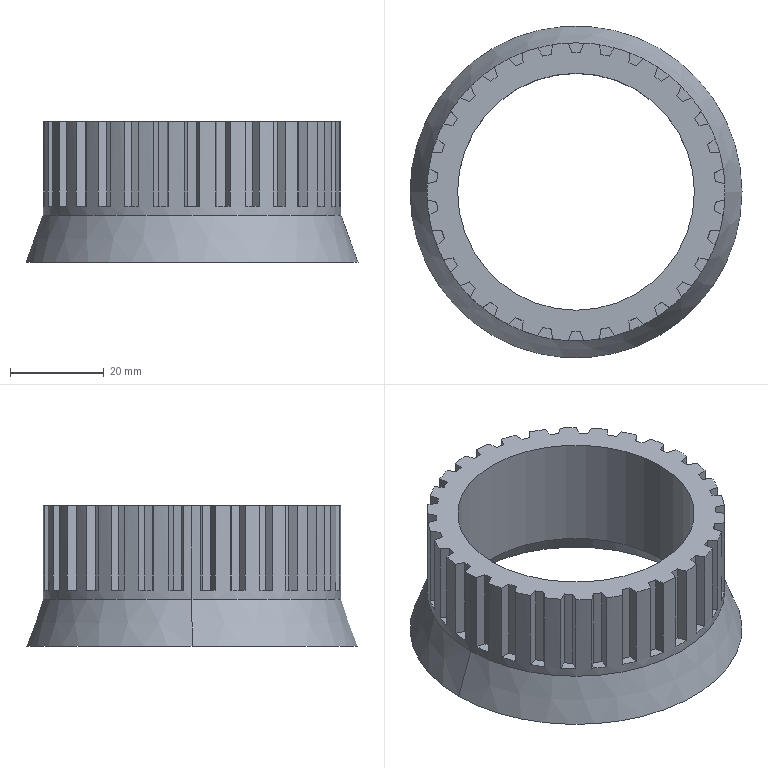Part | SolidWorks | features CirPattern 1, HoleWzd 1, ICE 1, Revolution 1 | 1 solid | 131 faces | box 70.779 x 70.779 x 30 mm | volume 32307 mm3 | plane 123 | cylinder 4 | cone 4 | commonest cylinder face diameters 50.5 x2 63.5 x2